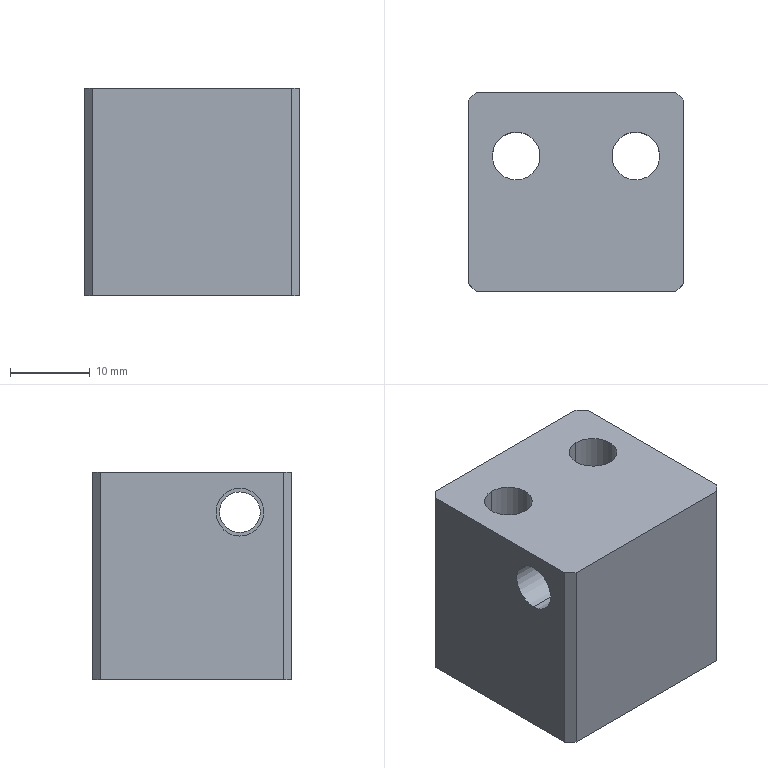Part | STEP file | J454-EBZ05-27-00-Part-1-2 | 1 solid | 36 faces | box 27 x 25 x 26 mm | volume 15181 mm3 | cylinder 18 | plane 14 | cone 4 | commonest cylinder face diameters 6 x8 2.5 x4 3 x4 5.1 x2
STEP:
#1=CARTESIAN_POINT('',(13.5,16.249,-3.3));
#2=VERTEX_POINT('',#1);
#3=CARTESIAN_POINT('',(14.75,17.,-3.3));
#4=VERTEX_POINT('',#3);
#5=CARTESIAN_POINT('',(14.75,17.,-3.3));
#6=DIRECTION('',(0.8572,0.515,0.));
#7=VECTOR('',#6,1000.);
#8=LINE('',#5,#7);
#9=EDGE_CURVE('',#2,#4,#8,.T.);
#10=ORIENTED_EDGE('',*,*,#9,.F.);
#11=CARTESIAN_POINT('',(12.25,17.,-3.3));
#12=VERTEX_POINT('',#11);
#13=CARTESIAN_POINT('',(12.25,17.,-3.3));
#14=DIRECTION('',(-0.8572,0.515,0.));
#15=VECTOR('',#14,1000.);
#16=LINE('',#13,#15);
#17=EDGE_CURVE('',#2,#12,#16,.T.);
#18=ORIENTED_EDGE('',*,*,#17,.T.);
#19=CARTESIAN_POINT('',(13.5,17.,-3.3));
#20=DIRECTION('',(0.,1.,0.));
#21=DIRECTION('',(1.,0.,0.));
#22=AXIS2_PLACEMENT_3D('',#19,#20,#21);
#23=CIRCLE('',#22,1.25);
#24=EDGE_CURVE('',#12,#4,#23,.T.);
#25=ORIENTED_EDGE('',*,*,#24,.T.);
#26=EDGE_LOOP('',(#10,#18,#25));
#27=FACE_OUTER_BOUND('',#26,.T.);
#28=CARTESIAN_POINT('',(13.5,17.,-3.3));
#29=DIRECTION('',(0.,1.,0.));
#30=DIRECTION('',(1.,0.,0.));
#31=AXIS2_PLACEMENT_3D('',#28,#29,#30);
#32=CONICAL_SURFACE('',#31,1.25,1.03);
#33=ADVANCED_FACE('',(#27),#32,.F.);
#34=ORIENTED_EDGE('',*,*,#24,.F.);
#35=CARTESIAN_POINT('',(12.25,19.,-3.3));
#36=VERTEX_POINT('',#35);
#37=CARTESIAN_POINT('',(12.25,25.,-3.3));
#38=DIRECTION('',(0.,1.,0.));
#39=VECTOR('',#38,1000.);
#40=LINE('',#37,#39);
#41=EDGE_CURVE('',#12,#36,#40,.T.);
#42=ORIENTED_EDGE('',*,*,#41,.T.);
#43=CARTESIAN_POINT('',(14.75,19.,-3.3));
#44=VERTEX_POINT('',#43);
#45=CARTESIAN_POINT('',(13.5,19.,-3.3));
#46=DIRECTION('',(0.,1.,0.));
#47=DIRECTION('',(1.,0.,0.));
#48=AXIS2_PLACEMENT_3D('',#45,#46,#47);
#49=CIRCLE('',#48,1.25);
#50=EDGE_CURVE('',#36,#44,#49,.T.);
#51=ORIENTED_EDGE('',*,*,#50,.T.);
#52=CARTESIAN_POINT('',(14.75,25.,-3.3));
#53=DIRECTION('',(0.,1.,0.));
#54=VECTOR('',#53,1000.);
#55=LINE('',#52,#54);
#56=EDGE_CURVE('',#4,#44,#55,.T.);
#57=ORIENTED_EDGE('',*,*,#56,.F.);
#58=EDGE_LOOP('',(#34,#42,#51,#57));
#59=FACE_OUTER_BOUND('',#58,.T.);
#60=CARTESIAN_POINT('',(13.5,25.,-3.3));
#61=DIRECTION('',(0.,1.,0.));
#62=DIRECTION('',(1.,0.,0.));
#63=AXIS2_PLACEMENT_3D('',#60,#61,#62);
#64=CYLINDRICAL_SURFACE('',#63,1.25);
#65=ADVANCED_FACE('',(#59),#64,.F.);
#66=CARTESIAN_POINT('',(12.,19.,-3.3));
#67=VERTEX_POINT('',#66);
#68=CARTESIAN_POINT('',(15.,19.,-3.3));
#69=VERTEX_POINT('',#68);
#70=CARTESIAN_POINT('',(13.5,19.,-3.3));
#71=DIRECTION('',(0.,1.,0.));
#72=DIRECTION('',(1.,0.,0.));
#73=AXIS2_PLACEMENT_3D('',#70,#71,#72);
#74=CIRCLE('',#73,1.5);
#75=EDGE_CURVE('',#67,#69,#74,.T.);
#76=ORIENTED_EDGE('',*,*,#75,.F.);
#77=CARTESIAN_POINT('',(12.,25.,-3.3));
#78=VERTEX_POINT('',#77);
#79=CARTESIAN_POINT('',(12.,25.,-3.3));
#80=DIRECTION('',(0.,1.,0.));
#81=VECTOR('',#80,1000.);
#82=LINE('',#79,#81);
#83=EDGE_CURVE('',#67,#78,#82,.T.);
#84=ORIENTED_EDGE('',*,*,#83,.T.);
#85=CARTESIAN_POINT('',(15.,25.,-3.3));
#86=VERTEX_POINT('',#85);
#87=CARTESIAN_POINT('',(13.5,25.,-3.3));
#88=DIRECTION('',(0.,1.,0.));
#89=DIRECTION('',(1.,0.,0.));
#90=AXIS2_PLACEMENT_3D('',#87,#88,#89);
#91=CIRCLE('',#90,1.5);
#92=EDGE_CURVE('',#78,#86,#91,.T.);
#93=ORIENTED_EDGE('',*,*,#92,.T.);
#94=CARTESIAN_POINT('',(15.,25.,-3.3));
#95=DIRECTION('',(0.,1.,0.));
#96=VECTOR('',#95,1000.);
#97=LINE('',#94,#96);
#98=EDGE_CURVE('',#69,#86,#97,.T.);
#99=ORIENTED_EDGE('',*,*,#98,.F.);
#100=EDGE_LOOP('',(#76,#84,#93,#99));
#101=FACE_OUTER_BOUND('',#100,.T.);
#102=CARTESIAN_POINT('',(13.5,25.,-3.3));
#103=DIRECTION('',(0.,1.,0.));
#104=DIRECTION('',(1.,0.,0.));
#105=AXIS2_PLACEMENT_3D('',#102,#103,#104);
#106=CYLINDRICAL_SURFACE('',#105,1.5);
#107=ADVANCED_FACE('',(#101),#106,.F.);
#108=CARTESIAN_POINT('',(13.5,16.249,9.3));
#109=VERTEX_POINT('',#108);
#110=CARTESIAN_POINT('',(14.75,17.,9.3));
#111=VERTEX_POINT('',#110);
#112=CARTESIAN_POINT('',(14.75,17.,9.3));
#113=DIRECTION('',(0.8572,0.515,0.));
#114=VECTOR('',#113,1000.);
#115=LINE('',#112,#114);
#116=EDGE_CURVE('',#109,#111,#115,.T.);
#117=ORIENTED_EDGE('',*,*,#116,.F.);
#118=CARTESIAN_POINT('',(12.25,17.,9.3));
#119=VERTEX_POINT('',#118);
#120=CARTESIAN_POINT('',(12.25,17.,9.3));
#121=DIRECTION('',(-0.8572,0.515,0.));
#122=VECTOR('',#121,1000.);
#123=LINE('',#120,#122);
#124=EDGE_CURVE('',#109,#119,#123,.T.);
#125=ORIENTED_EDGE('',*,*,#124,.T.);
#126=CARTESIAN_POINT('',(13.5,17.,9.3));
#127=DIRECTION('',(0.,1.,0.));
#128=DIRECTION('',(1.,0.,0.));
#129=AXIS2_PLACEMENT_3D('',#126,#127,#128);
#130=CIRCLE('',#129,1.25);
#131=EDGE_CURVE('',#119,#111,#130,.T.);
#132=ORIENTED_EDGE('',*,*,#131,.T.);
#133=EDGE_LOOP('',(#117,#125,#132));
#134=FACE_OUTER_BOUND('',#133,.T.);
#135=CARTESIAN_POINT('',(13.5,17.,9.3));
#136=DIRECTION('',(0.,1.,0.));
#137=DIRECTION('',(1.,0.,0.));
#138=AXIS2_PLACEMENT_3D('',#135,#136,#137);
#139=CONICAL_SURFACE('',#138,1.25,1.03);
#140=ADVANCED_FACE('',(#134),#139,.F.);
#141=ORIENTED_EDGE('',*,*,#131,.F.);
#142=CARTESIAN_POINT('',(12.25,19.,9.3));
#143=VERTEX_POINT('',#142);
#144=CARTESIAN_POINT('',(12.25,25.,9.3));
#145=DIRECTION('',(0.,1.,0.));
#146=VECTOR('',#145,1000.);
#147=LINE('',#144,#146);
#148=EDGE_CURVE('',#119,#143,#147,.T.);
#149=ORIENTED_EDGE('',*,*,#148,.T.);
#150=CARTESIAN_POINT('',(14.75,19.,9.3));
#151=VERTEX_POINT('',#150);
#152=CARTESIAN_POINT('',(13.5,19.,9.3));
#153=DIRECTION('',(0.,1.,0.));
#154=DIRECTION('',(1.,0.,0.));
#155=AXIS2_PLACEMENT_3D('',#152,#153,#154);
#156=CIRCLE('',#155,1.25);
#157=EDGE_CURVE('',#143,#151,#156,.T.);
#158=ORIENTED_EDGE('',*,*,#157,.T.);
#159=CARTESIAN_POINT('',(14.75,25.,9.3));
#160=DIRECTION('',(0.,1.,0.));
#161=VECTOR('',#160,1000.);
#162=LINE('',#159,#161);
#163=EDGE_CURVE('',#111,#151,#162,.T.);
#164=ORIENTED_EDGE('',*,*,#163,.F.);
#165=EDGE_LOOP('',(#141,#149,#158,#164));
#166=FACE_OUTER_BOUND('',#165,.T.);
#167=CARTESIAN_POINT('',(13.5,25.,9.3));
#168=DIRECTION('',(0.,1.,0.));
#169=DIRECTION('',(1.,0.,0.));
#170=AXIS2_PLACEMENT_3D('',#167,#168,#169);
#171=CYLINDRICAL_SURFACE('',#170,1.25);
#172=ADVANCED_FACE('',(#166),#171,.F.);
#173=CARTESIAN_POINT('',(12.,19.,9.3));
#174=VERTEX_POINT('',#173);
#175=CARTESIAN_POINT('',(15.,19.,9.3));
#176=VERTEX_POINT('',#175);
#177=CARTESIAN_POINT('',(13.5,19.,9.3));
#178=DIRECTION('',(0.,1.,0.));
#179=DIRECTION('',(1.,0.,0.));
#180=AXIS2_PLACEMENT_3D('',#177,#178,#179);
#181=CIRCLE('',#180,1.5);
#182=EDGE_CURVE('',#174,#176,#181,.T.);
#183=ORIENTED_EDGE('',*,*,#182,.F.);
#184=CARTESIAN_POINT('',(12.,25.,9.3));
#185=VERTEX_POINT('',#184);
#186=CARTESIAN_POINT('',(12.,25.,9.3));
#187=DIRECTION('',(0.,1.,0.));
#188=VECTOR('',#187,1000.);
#189=LINE('',#186,#188);
#190=EDGE_CURVE('',#174,#185,#189,.T.);
#191=ORIENTED_EDGE('',*,*,#190,.T.);
#192=CARTESIAN_POINT('',(15.,25.,9.3));
#193=VERTEX_POINT('',#192);
#194=CARTESIAN_POINT('',(13.5,25.,9.3));
#195=DIRECTION('',(0.,1.,0.));
#196=DIRECTION('',(1.,0.,0.));
#197=AXIS2_PLACEMENT_3D('',#194,#195,#196);
#198=CIRCLE('',#197,1.5);
#199=EDGE_CURVE('',#185,#193,#198,.T.);
#200=ORIENTED_EDGE('',*,*,#199,.T.);
#201=CARTESIAN_POINT('',(15.,25.,9.3));
#202=DIRECTION('',(0.,1.,0.));
#203=VECTOR('',#202,1000.);
#204=LINE('',#201,#203);
#205=EDGE_CURVE('',#176,#193,#204,.T.);
#206=ORIENTED_EDGE('',*,*,#205,.F.);
#207=EDGE_LOOP('',(#183,#191,#200,#206));
#208=FACE_OUTER_BOUND('',#207,.T.);
#209=CARTESIAN_POINT('',(13.5,25.,9.3));
#210=DIRECTION('',(0.,1.,0.));
#211=DIRECTION('',(1.,0.,0.));
#212=AXIS2_PLACEMENT_3D('',#209,#210,#211);
#213=CYLINDRICAL_SURFACE('',#212,1.5);
#214=ADVANCED_FACE('',(#208),#213,.F.);
#215=CARTESIAN_POINT('',(12.,6.5,8.));
#216=VERTEX_POINT('',#215);
#217=CARTESIAN_POINT('',(12.,6.5,14.));
#218=VERTEX_POINT('',#217);
#219=CARTESIAN_POINT('',(12.,6.5,11.));
#220=DIRECTION('',(-1.,0.,0.));
#221=DIRECTION('',(0.,0.,1.));
#222=AXIS2_PLACEMENT_3D('',#219,#220,#221);
#223=CIRCLE('',#222,3.);
#224=EDGE_CURVE('',#216,#218,#223,.T.);
#225=ORIENTED_EDGE('',*,*,#224,.F.);
#226=CARTESIAN_POINT('',(0.,6.5,8.));
#227=VERTEX_POINT('',#226);
#228=CARTESIAN_POINT('',(0.,6.5,8.));
#229=DIRECTION('',(-1.,0.,0.));
#230=VECTOR('',#229,1000.);
#231=LINE('',#228,#230);
#232=EDGE_CURVE('',#216,#227,#231,.T.);
#233=ORIENTED_EDGE('',*,*,#232,.T.);
#234=CARTESIAN_POINT('',(0.,6.5,14.));
#235=VERTEX_POINT('',#234);
#236=CARTESIAN_POINT('',(0.,6.5,11.));
#237=DIRECTION('',(-1.,0.,0.));
#238=DIRECTION('',(0.,0.,1.));
#239=AXIS2_PLACEMENT_3D('',#236,#237,#238);
#240=CIRCLE('',#239,3.);
#241=EDGE_CURVE('',#227,#235,#240,.T.);
#242=ORIENTED_EDGE('',*,*,#241,.T.);
#243=CARTESIAN_POINT('',(0.,6.5,14.));
#244=DIRECTION('',(-1.,0.,0.));
#245=VECTOR('',#244,1000.);
#246=LINE('',#243,#245);
#247=EDGE_CURVE('',#218,#235,#246,.T.);
#248=ORIENTED_EDGE('',*,*,#247,.F.);
#249=EDGE_LOOP('',(#225,#233,#242,#248));
#250=FACE_OUTER_BOUND('',#249,.T.);
#251=CARTESIAN_POINT('',(0.,6.5,11.));
#252=DIRECTION('',(-1.,0.,0.));
#253=DIRECTION('',(0.,0.,1.));
#254=AXIS2_PLACEMENT_3D('',#251,#252,#253);
#255=CYLINDRICAL_SURFACE('',#254,3.);
#256=ADVANCED_FACE('',(#250),#255,.F.);
#257=CARTESIAN_POINT('',(12.,6.5,13.55));
#258=VERTEX_POINT('',#257);
#259=CARTESIAN_POINT('',(12.,6.5,8.45));
#260=VERTEX_POINT('',#259);
#261=CARTESIAN_POINT('',(12.,6.5,11.));
#262=DIRECTION('',(-1.,0.,0.));
#263=DIRECTION('',(0.,0.,1.));
#264=AXIS2_PLACEMENT_3D('',#261,#262,#263);
#265=CIRCLE('',#264,2.55);
#266=EDGE_CURVE('',#258,#260,#265,.T.);
#267=ORIENTED_EDGE('',*,*,#266,.T.);
#268=CARTESIAN_POINT('',(15.,6.5,8.45));
#269=VERTEX_POINT('',#268);
#270=CARTESIAN_POINT('',(27.,6.5,8.45));
#271=DIRECTION('',(1.,0.,0.));
#272=VECTOR('',#271,1000.);
#273=LINE('',#270,#272);
#274=EDGE_CURVE('',#260,#269,#273,.T.);
#275=ORIENTED_EDGE('',*,*,#274,.T.);
#276=CARTESIAN_POINT('',(15.,6.5,13.55));
#277=VERTEX_POINT('',#276);
#278=CARTESIAN_POINT('',(15.,6.5,11.));
#279=DIRECTION('',(1.,0.,0.));
#280=DIRECTION('',(0.,0.,1.));
#281=AXIS2_PLACEMENT_3D('',#278,#279,#280);
#282=CIRCLE('',#281,2.55);
#283=EDGE_CURVE('',#269,#277,#282,.T.);
#284=ORIENTED_EDGE('',*,*,#283,.T.);
#285=CARTESIAN_POINT('',(27.,6.5,13.55));
#286=DIRECTION('',(1.,0.,0.));
#287=VECTOR('',#286,1000.);
#288=LINE('',#285,#287);
#289=EDGE_CURVE('',#258,#277,#288,.T.);
#290=ORIENTED_EDGE('',*,*,#289,.F.);
#291=EDGE_LOOP('',(#267,#275,#284,#290));
#292=FACE_OUTER_BOUND('',#291,.T.);
#293=CARTESIAN_POINT('',(27.,6.5,11.));
#294=DIRECTION('',(1.,0.,0.));
#295=DIRECTION('',(0.,0.,1.));
#296=AXIS2_PLACEMENT_3D('',#293,#294,#295);
#297=CYLINDRICAL_SURFACE('',#296,2.55);
#298=ADVANCED_FACE('',(#292),#297,.F.);
#299=CARTESIAN_POINT('',(15.,6.5,8.));
#300=VERTEX_POINT('',#299);
#301=CARTESIAN_POINT('',(15.,6.5,14.));
#302=VERTEX_POINT('',#301);
#303=CARTESIAN_POINT('',(15.,6.5,11.));
#304=DIRECTION('',(1.,0.,0.));
#305=DIRECTION('',(0.,0.,1.));
#306=AXIS2_PLACEMENT_3D('',#303,#304,#305);
#307=CIRCLE('',#306,3.);
#308=EDGE_CURVE('',#300,#302,#307,.T.);
#309=ORIENTED_EDGE('',*,*,#308,.F.);
#310=CARTESIAN_POINT('',(27.,6.5,8.));
#311=VERTEX_POINT('',#310);
#312=CARTESIAN_POINT('',(27.,6.5,8.));
#313=DIRECTION('',(1.,0.,0.));
#314=VECTOR('',#313,1000.);
#315=LINE('',#312,#314);
#316=EDGE_CURVE('',#300,#311,#315,.T.);
#317=ORIENTED_EDGE('',*,*,#316,.T.);
#318=CARTESIAN_POINT('',(27.,6.5,14.));
#319=VERTEX_POINT('',#318);
#320=CARTESIAN_POINT('',(27.,6.5,11.));
#321=DIRECTION('',(1.,0.,0.));
#322=DIRECTION('',(0.,0.,1.));
#323=AXIS2_PLACEMENT_3D('',#320,#321,#322);
#324=CIRCLE('',#323,3.);
#325=EDGE_CURVE('',#311,#319,#324,.T.);
#326=ORIENTED_EDGE('',*,*,#325,.T.);
#327=CARTESIAN_POINT('',(27.,6.5,14.));
#328=DIRECTION('',(1.,0.,0.));
#329=VECTOR('',#328,1000.);
#330=LINE('',#327,#329);
#331=EDGE_CURVE('',#302,#319,#330,.T.);
#332=ORIENTED_EDGE('',*,*,#331,.F.);
#333=EDGE_LOOP('',(#309,#317,#326,#332));
#334=FACE_OUTER_BOUND('',#333,.T.);
#335=CARTESIAN_POINT('',(27.,6.5,11.));
#336=DIRECTION('',(1.,0.,0.));
#337=DIRECTION('',(0.,0.,1.));
#338=AXIS2_PLACEMENT_3D('',#335,#336,#337);
#339=CYLINDRICAL_SURFACE('',#338,3.);
#340=ADVANCED_FACE('',(#334),#339,.F.);
#341=CARTESIAN_POINT('',(6.,20.,16.));
#342=VERTEX_POINT('',#341);
#343=CARTESIAN_POINT('',(6.,14.,16.));
#344=VERTEX_POINT('',#343);
#345=CARTESIAN_POINT('',(6.,17.,16.));
#346=DIRECTION('',(0.,0.,-1.));
#347=DIRECTION('',(0.,-1.,0.));
#348=AXIS2_PLACEMENT_3D('',#345,#346,#347);
#349=CIRCLE('',#348,3.);
#350=EDGE_CURVE('',#342,#344,#349,.T.);
#351=ORIENTED_EDGE('',*,*,#350,.F.);
#352=CARTESIAN_POINT('',(6.,20.,-10.));
#353=VERTEX_POINT('',#352);
#354=CARTESIAN_POINT('',(6.,20.,16.));
#355=DIRECTION('',(0.,0.,-1.));
#356=VECTOR('',#355,1000.);
#357=LINE('',#354,#356);
#358=EDGE_CURVE('',#342,#353,#357,.T.);
#359=ORIENTED_EDGE('',*,*,#358,.T.);
#360=CARTESIAN_POINT('',(6.,14.,-10.));
#361=VERTEX_POINT('',#360);
#362=CARTESIAN_POINT('',(6.,17.,-10.));
#363=DIRECTION('',(0.,0.,1.));
#364=DIRECTION('',(0.,1.,0.));
#365=AXIS2_PLACEMENT_3D('',#362,#363,#364);
#366=CIRCLE('',#365,3.);
#367=EDGE_CURVE('',#361,#353,#366,.T.);
#368=ORIENTED_EDGE('',*,*,#367,.F.);
#369=CARTESIAN_POINT('',(6.,14.,16.));
#370=DIRECTION('',(0.,0.,-1.));
#371=VECTOR('',#370,1000.);
#372=LINE('',#369,#371);
#373=EDGE_CURVE('',#344,#361,#372,.T.);
#374=ORIENTED_EDGE('',*,*,#373,.F.);
#375=EDGE_LOOP('',(#351,#359,#368,#374));
#376=FACE_OUTER_BOUND('',#375,.T.);
#377=CARTESIAN_POINT('',(6.,17.,16.));
#378=DIRECTION('',(0.,0.,-1.));
#379=DIRECTION('',(0.,-1.,0.));
#380=AXIS2_PLACEMENT_3D('',#377,#378,#379);
#381=CYLINDRICAL_SURFACE('',#380,3.);
#382=ADVANCED_FACE('',(#376),#381,.F.);
#383=CARTESIAN_POINT('',(21.,20.,16.));
#384=VERTEX_POINT('',#383);
#385=CARTESIAN_POINT('',(21.,14.,16.));
#386=VERTEX_POINT('',#385);
#387=CARTESIAN_POINT('',(21.,17.,16.));
#388=DIRECTION('',(0.,0.,-1.));
#389=DIRECTION('',(0.,-1.,0.));
#390=AXIS2_PLACEMENT_3D('',#387,#388,#389);
#391=CIRCLE('',#390,3.);
#392=EDGE_CURVE('',#384,#386,#391,.T.);
#393=ORIENTED_EDGE('',*,*,#392,.F.);
#394=CARTESIAN_POINT('',(21.,20.,-10.));
#395=VERTEX_POINT('',#394);
#396=CARTESIAN_POINT('',(21.,20.,16.));
#397=DIRECTION('',(0.,0.,-1.));
#398=VECTOR('',#397,1000.);
#399=LINE('',#396,#398);
#400=EDGE_CURVE('',#384,#395,#399,.T.);
#401=ORIENTED_EDGE('',*,*,#400,.T.);
#402=CARTESIAN_POINT('',(21.,14.,-10.));
#403=VERTEX_POINT('',#402);
#404=CARTESIAN_POINT('',(21.,17.,-10.));
#405=DIRECTION('',(0.,0.,1.));
#406=DIRECTION('',(0.,1.,0.));
#407=AXIS2_PLACEMENT_3D('',#404,#405,#406);
#408=CIRCLE('',#407,3.);
#409=EDGE_CURVE('',#403,#395,#408,.T.);
#410=ORIENTED_EDGE('',*,*,#409,.F.);
#411=CARTESIAN_POINT('',(21.,14.,16.));
#412=DIRECTION('',(0.,0.,-1.));
#413=VECTOR('',#412,1000.);
#414=LINE('',#411,#413);
#415=EDGE_CURVE('',#386,#403,#414,.T.);
#416=ORIENTED_EDGE('',*,*,#415,.F.);
#417=EDGE_LOOP('',(#393,#401,#410,#416));
#418=FACE_OUTER_BOUND('',#417,.T.);
#419=CARTESIAN_POINT('',(21.,17.,16.));
#420=DIRECTION('',(0.,0.,-1.));
#421=DIRECTION('',(0.,-1.,0.));
#422=AXIS2_PLACEMENT_3D('',#419,#420,#421);
#423=CYLINDRICAL_SURFACE('',#422,3.);
#424=ADVANCED_FACE('',(#418),#423,.F.);
#425=CARTESIAN_POINT('',(6.,17.,16.));
#426=DIRECTION('',(0.,0.,-1.));
#427=DIRECTION('',(0.,-1.,0.));
#428=AXIS2_PLACEMENT_3D('',#425,#426,#427);
#429=CIRCLE('',#428,3.);
#430=EDGE_CURVE('',#344,#342,#429,.T.);
#431=ORIENTED_EDGE('',*,*,#430,.T.);
#432=ORIENTED_EDGE('',*,*,#350,.T.);
#433=EDGE_LOOP('',(#431,#432));
#434=FACE_BOUND('',#433,.T.);
#435=CARTESIAN_POINT('',(21.,17.,16.));
#436=DIRECTION('',(0.,0.,-1.));
#437=DIRECTION('',(0.,-1.,0.));
#438=AXIS2_PLACEMENT_3D('',#435,#436,#437);
#439=CIRCLE('',#438,3.);
#440=EDGE_CURVE('',#386,#384,#439,.T.);
#441=ORIENTED_EDGE('',*,*,#440,.T.);
#442=ORIENTED_EDGE('',*,*,#392,.T.);
#443=EDGE_LOOP('',(#441,#442));
#444=FACE_BOUND('',#443,.T.);
#445=CARTESIAN_POINT('',(26.,0.,16.));
#446=VERTEX_POINT('',#445);
#447=CARTESIAN_POINT('',(1.,0.,16.));
#448=VERTEX_POINT('',#447);
#449=CARTESIAN_POINT('',(13.5,0.,16.));
#450=DIRECTION('',(-1.,0.,0.));
#451=VECTOR('',#450,1000.);
#452=LINE('',#449,#451);
#453=EDGE_CURVE('',#446,#448,#452,.T.);
#454=ORIENTED_EDGE('',*,*,#453,.F.);
#455=CARTESIAN_POINT('',(27.,1.,16.));
#456=VERTEX_POINT('',#455);
#457=CARTESIAN_POINT('',(26.,0.,16.));
#458=DIRECTION('',(0.7071,0.7071,0.));
#459=VECTOR('',#458,1000.);
#460=LINE('',#457,#459);
#461=EDGE_CURVE('',#446,#456,#460,.T.);
#462=ORIENTED_EDGE('',*,*,#461,.T.);
#463=CARTESIAN_POINT('',(27.,24.,16.));
#464=VERTEX_POINT('',#463);
#465=CARTESIAN_POINT('',(27.,12.5,16.));
#466=DIRECTION('',(0.,-1.,0.));
#467=VECTOR('',#466,1000.);
#468=LINE('',#465,#467);
#469=EDGE_CURVE('',#464,#456,#468,.T.);
#470=ORIENTED_EDGE('',*,*,#469,.F.);
#471=CARTESIAN_POINT('',(26.,25.,16.));
#472=VERTEX_POINT('',#471);
#473=CARTESIAN_POINT('',(26.,25.,16.));
#474=DIRECTION('',(-0.7071,0.7071,0.));
#475=VECTOR('',#474,1000.);
#476=LINE('',#473,#475);
#477=EDGE_CURVE('',#464,#472,#476,.T.);
#478=ORIENTED_EDGE('',*,*,#477,.T.);
#479=CARTESIAN_POINT('',(1.,25.,16.));
#480=VERTEX_POINT('',#479);
#481=CARTESIAN_POINT('',(13.5,25.,16.));
#482=DIRECTION('',(1.,0.,0.));
#483=VECTOR('',#482,1000.);
#484=LINE('',#481,#483);
#485=EDGE_CURVE('',#480,#472,#484,.T.);
#486=ORIENTED_EDGE('',*,*,#485,.F.);
#487=CARTESIAN_POINT('',(0.,24.,16.));
#488=VERTEX_POINT('',#487);
#489=CARTESIAN_POINT('',(1.,25.,16.));
#490=DIRECTION('',(-0.7071,-0.7071,0.));
#491=VECTOR('',#490,1000.);
#492=LINE('',#489,#491);
#493=EDGE_CURVE('',#480,#488,#492,.T.);
#494=ORIENTED_EDGE('',*,*,#493,.T.);
#495=CARTESIAN_POINT('',(0.,1.,16.));
#496=VERTEX_POINT('',#495);
#497=CARTESIAN_POINT('',(0.,12.5,16.));
#498=DIRECTION('',(0.,1.,0.));
#499=VECTOR('',#498,1000.);
#500=LINE('',#497,#499);
#501=EDGE_CURVE('',#496,#488,#500,.T.);
#502=ORIENTED_EDGE('',*,*,#501,.F.);
#503=CARTESIAN_POINT('',(1.,0.,16.));
#504=DIRECTION('',(0.7071,-0.7071,0.));
#505=VECTOR('',#504,1000.);
#506=LINE('',#503,#505);
#507=EDGE_CURVE('',#496,#448,#506,.T.);
#508=ORIENTED_EDGE('',*,*,#507,.T.);
#509=EDGE_LOOP('',(#454,#462,#470,#478,#486,#494,#502,#508));
#510=FACE_OUTER_BOUND('',#509,.T.);
#511=CARTESIAN_POINT('',(13.5,12.5,16.));
#512=DIRECTION('',(0.,0.,1.));
#513=DIRECTION('',(0.,1.,0.));
#514=AXIS2_PLACEMENT_3D('',#511,#512,#513);
#515=PLANE('',#514);
#516=ADVANCED_FACE('',(#434,#444,#510),#515,.T.);
#517=CARTESIAN_POINT('',(27.,6.5,11.));
#518=DIRECTION('',(1.,0.,0.));
#519=DIRECTION('',(0.,0.,1.));
#520=AXIS2_PLACEMENT_3D('',#517,#518,#519);
#521=CIRCLE('',#520,3.);
#522=EDGE_CURVE('',#319,#311,#521,.T.);
#523=ORIENTED_EDGE('',*,*,#522,.F.);
#524=ORIENTED_EDGE('',*,*,#325,.F.);
#525=EDGE_LOOP('',(#523,#524));
#526=FACE_BOUND('',#525,.T.);
#527=ORIENTED_EDGE('',*,*,#469,.T.);
#528=CARTESIAN_POINT('',(27.,1.,-10.));
#529=VERTEX_POINT('',#528);
#530=CARTESIAN_POINT('',(27.,1.,-10.));
#531=DIRECTION('',(0.,0.,-1.));
#532=VECTOR('',#531,1000.);
#533=LINE('',#530,#532);
#534=EDGE_CURVE('',#456,#529,#533,.T.);
#535=ORIENTED_EDGE('',*,*,#534,.T.);
#536=CARTESIAN_POINT('',(27.,24.,-10.));
#537=VERTEX_POINT('',#536);
#538=CARTESIAN_POINT('',(27.,12.5,-10.));
#539=DIRECTION('',(0.,1.,0.));
#540=VECTOR('',#539,1000.);
#541=LINE('',#538,#540);
#542=EDGE_CURVE('',#529,#537,#541,.T.);
#543=ORIENTED_EDGE('',*,*,#542,.T.);
#544=CARTESIAN_POINT('',(27.,24.,-10.));
#545=DIRECTION('',(0.,0.,1.));
#546=VECTOR('',#545,1000.);
#547=LINE('',#544,#546);
#548=EDGE_CURVE('',#537,#464,#547,.T.);
#549=ORIENTED_EDGE('',*,*,#548,.T.);
#550=EDGE_LOOP('',(#527,#535,#543,#549));
#551=FACE_OUTER_BOUND('',#550,.T.);
#552=CARTESIAN_POINT('',(27.,12.5,-10.));
#553=DIRECTION('',(1.,0.,0.));
#554=DIRECTION('',(0.,0.,-1.));
#555=AXIS2_PLACEMENT_3D('',#552,#553,#554);
#556=PLANE('',#555);
#557=ADVANCED_FACE('',(#526,#551),#556,.T.);
#558=CARTESIAN_POINT('',(1.,0.,-10.));
#559=VERTEX_POINT('',#558);
#560=CARTESIAN_POINT('',(26.,0.,-10.));
#561=VERTEX_POINT('',#560);
#562=CARTESIAN_POINT('',(13.5,0.,-10.));
#563=DIRECTION('',(1.,0.,0.));
#564=VECTOR('',#563,1000.);
#565=LINE('',#562,#564);
#566=EDGE_CURVE('',#559,#561,#565,.T.);
#567=ORIENTED_EDGE('',*,*,#566,.T.);
#568=CARTESIAN_POINT('',(26.,0.,-10.));
#569=DIRECTION('',(0.,0.,1.));
#570=VECTOR('',#569,1000.);
#571=LINE('',#568,#570);
#572=EDGE_CURVE('',#561,#446,#571,.T.);
#573=ORIENTED_EDGE('',*,*,#572,.T.);
#574=ORIENTED_EDGE('',*,*,#453,.T.);
#575=CARTESIAN_POINT('',(1.,0.,-10.));
#576=DIRECTION('',(0.,0.,-1.));
#577=VECTOR('',#576,1000.);
#578=LINE('',#575,#577);
#579=EDGE_CURVE('',#448,#559,#578,.T.);
#580=ORIENTED_EDGE('',*,*,#579,.T.);
#581=EDGE_LOOP('',(#567,#573,#574,#580));
#582=FACE_OUTER_BOUND('',#581,.T.);
#583=CARTESIAN_POINT('',(13.5,0.,-10.));
#584=DIRECTION('',(0.,-1.,0.));
#585=DIRECTION('',(0.,0.,1.));
#586=AXIS2_PLACEMENT_3D('',#583,#584,#585);
#587=PLANE('',#586);
#588=ADVANCED_FACE('',(#582),#587,.T.);
#589=CARTESIAN_POINT('',(0.,6.5,11.));
#590=DIRECTION('',(-1.,0.,0.));
#591=DIRECTION('',(0.,0.,1.));
#592=AXIS2_PLACEMENT_3D('',#589,#590,#591);
#593=CIRCLE('',#592,3.);
#594=EDGE_CURVE('',#235,#227,#593,.T.);
#595=ORIENTED_EDGE('',*,*,#594,.F.);
#596=ORIENTED_EDGE('',*,*,#241,.F.);
#597=EDGE_LOOP('',(#595,#596));
#598=FACE_BOUND('',#597,.T.);
#599=CARTESIAN_POINT('',(0.,24.,-10.));
#600=VERTEX_POINT('',#599);
#601=CARTESIAN_POINT('',(0.,1.,-10.));
#602=VERTEX_POINT('',#601);
#603=CARTESIAN_POINT('',(0.,12.5,-10.));
#604=DIRECTION('',(0.,-1.,0.));
#605=VECTOR('',#604,1000.);
#606=LINE('',#603,#605);
#607=EDGE_CURVE('',#600,#602,#606,.T.);
#608=ORIENTED_EDGE('',*,*,#607,.T.);
#609=CARTESIAN_POINT('',(0.,1.,-10.));
#610=DIRECTION('',(0.,0.,1.));
#611=VECTOR('',#610,1000.);
#612=LINE('',#609,#611);
#613=EDGE_CURVE('',#602,#496,#612,.T.);
#614=ORIENTED_EDGE('',*,*,#613,.T.);
#615=ORIENTED_EDGE('',*,*,#501,.T.);
#616=CARTESIAN_POINT('',(0.,24.,-10.));
#617=DIRECTION('',(0.,0.,-1.));
#618=VECTOR('',#617,1000.);
#619=LINE('',#616,#618);
#620=EDGE_CURVE('',#488,#600,#619,.T.);
#621=ORIENTED_EDGE('',*,*,#620,.T.);
#622=EDGE_LOOP('',(#608,#614,#615,#621));
#623=FACE_OUTER_BOUND('',#622,.T.);
#624=CARTESIAN_POINT('',(0.,12.5,-10.));
#625=DIRECTION('',(-1.,0.,0.));
#626=DIRECTION('',(0.,0.,1.));
#627=AXIS2_PLACEMENT_3D('',#624,#625,#626);
#628=PLANE('',#627);
#629=ADVANCED_FACE('',(#598,#623),#628,.T.);
#630=ORIENTED_EDGE('',*,*,#367,.T.);
#631=CARTESIAN_POINT('',(6.,17.,-10.));
#632=DIRECTION('',(0.,0.,1.));
#633=DIRECTION('',(0.,1.,0.));
#634=AXIS2_PLACEMENT_3D('',#631,#632,#633);
#635=CIRCLE('',#634,3.);
#636=EDGE_CURVE('',#353,#361,#635,.T.);
#637=ORIENTED_EDGE('',*,*,#636,.T.);
#638=EDGE_LOOP('',(#630,#637));
#639=FACE_BOUND('',#638,.T.);
#640=ORIENTED_EDGE('',*,*,#409,.T.);
#641=CARTESIAN_POINT('',(21.,17.,-10.));
#642=DIRECTION('',(0.,0.,1.));
#643=DIRECTION('',(0.,1.,0.));
#644=AXIS2_PLACEMENT_3D('',#641,#642,#643);
#645=CIRCLE('',#644,3.);
#646=EDGE_CURVE('',#395,#403,#645,.T.);
#647=ORIENTED_EDGE('',*,*,#646,.T.);
#648=EDGE_LOOP('',(#640,#647));
#649=FACE_BOUND('',#648,.T.);
#650=ORIENTED_EDGE('',*,*,#542,.F.);
#651=CARTESIAN_POINT('',(26.,0.,-10.));
#652=DIRECTION('',(-0.7071,-0.7071,0.));
#653=VECTOR('',#652,1000.);
#654=LINE('',#651,#653);
#655=EDGE_CURVE('',#529,#561,#654,.T.);
#656=ORIENTED_EDGE('',*,*,#655,.T.);
#657=ORIENTED_EDGE('',*,*,#566,.F.);
#658=CARTESIAN_POINT('',(1.,0.,-10.));
#659=DIRECTION('',(-0.7071,0.7071,0.));
#660=VECTOR('',#659,1000.);
#661=LINE('',#658,#660);
#662=EDGE_CURVE('',#559,#602,#661,.T.);
#663=ORIENTED_EDGE('',*,*,#662,.T.);
#664=ORIENTED_EDGE('',*,*,#607,.F.);
#665=CARTESIAN_POINT('',(1.,25.,-10.));
#666=VERTEX_POINT('',#665);
#667=CARTESIAN_POINT('',(1.,25.,-10.));
#668=DIRECTION('',(0.7071,0.7071,0.));
#669=VECTOR('',#668,1000.);
#670=LINE('',#667,#669);
#671=EDGE_CURVE('',#600,#666,#670,.T.);
#672=ORIENTED_EDGE('',*,*,#671,.T.);
#673=CARTESIAN_POINT('',(26.,25.,-10.));
#674=VERTEX_POINT('',#673);
#675=CARTESIAN_POINT('',(13.5,25.,-10.));
#676=DIRECTION('',(-1.,0.,0.));
#677=VECTOR('',#676,1000.);
#678=LINE('',#675,#677);
#679=EDGE_CURVE('',#674,#666,#678,.T.);
#680=ORIENTED_EDGE('',*,*,#679,.F.);
#681=CARTESIAN_POINT('',(26.,25.,-10.));
#682=DIRECTION('',(0.7071,-0.7071,0.));
#683=VECTOR('',#682,1000.);
#684=LINE('',#681,#683);
#685=EDGE_CURVE('',#674,#537,#684,.T.);
#686=ORIENTED_EDGE('',*,*,#685,.T.);
#687=EDGE_LOOP('',(#650,#656,#657,#663,#664,#672,#680,#686));
#688=FACE_OUTER_BOUND('',#687,.T.);
#689=CARTESIAN_POINT('',(13.5,12.5,-10.));
#690=DIRECTION('',(0.,0.,-1.));
#691=DIRECTION('',(0.,-1.,0.));
#692=AXIS2_PLACEMENT_3D('',#689,#690,#691);
#693=PLANE('',#692);
#694=ADVANCED_FACE('',(#639,#649,#688),#693,.T.);
#695=CARTESIAN_POINT('',(13.5,25.,-3.3));
#696=DIRECTION('',(0.,1.,0.));
#697=DIRECTION('',(1.,0.,0.));
#698=AXIS2_PLACEMENT_3D('',#695,#696,#697);
#699=CIRCLE('',#698,1.5);
#700=EDGE_CURVE('',#86,#78,#699,.T.);
#701=ORIENTED_EDGE('',*,*,#700,.F.);
#702=ORIENTED_EDGE('',*,*,#92,.F.);
#703=EDGE_LOOP('',(#701,#702));
#704=FACE_BOUND('',#703,.T.);
#705=CARTESIAN_POINT('',(13.5,25.,9.3));
#706=DIRECTION('',(0.,1.,0.));
#707=DIRECTION('',(1.,0.,0.));
#708=AXIS2_PLACEMENT_3D('',#705,#706,#707);
#709=CIRCLE('',#708,1.5);
#710=EDGE_CURVE('',#193,#185,#709,.T.);
#711=ORIENTED_EDGE('',*,*,#710,.F.);
#712=ORIENTED_EDGE('',*,*,#199,.F.);
#713=EDGE_LOOP('',(#711,#712));
#714=FACE_BOUND('',#713,.T.);
#715=ORIENTED_EDGE('',*,*,#679,.T.);
#716=CARTESIAN_POINT('',(1.,25.,-10.));
#717=DIRECTION('',(0.,0.,1.));
#718=VECTOR('',#717,1000.);
#719=LINE('',#716,#718);
#720=EDGE_CURVE('',#666,#480,#719,.T.);
#721=ORIENTED_EDGE('',*,*,#720,.T.);
#722=ORIENTED_EDGE('',*,*,#485,.T.);
#723=CARTESIAN_POINT('',(26.,25.,-10.));
#724=DIRECTION('',(0.,0.,-1.));
#725=VECTOR('',#724,1000.);
#726=LINE('',#723,#725);
#727=EDGE_CURVE('',#472,#674,#726,.T.);
#728=ORIENTED_EDGE('',*,*,#727,.T.);
#729=EDGE_LOOP('',(#715,#721,#722,#728));
#730=FACE_OUTER_BOUND('',#729,.T.);
#731=CARTESIAN_POINT('',(13.5,25.,-10.));
#732=DIRECTION('',(0.,1.,0.));
#733=DIRECTION('',(0.,0.,-1.));
#734=AXIS2_PLACEMENT_3D('',#731,#732,#733);
#735=PLANE('',#734);
#736=ADVANCED_FACE('',(#704,#714,#730),#735,.T.);
#737=ORIENTED_EDGE('',*,*,#400,.F.);
#738=ORIENTED_EDGE('',*,*,#440,.F.);
#739=ORIENTED_EDGE('',*,*,#415,.T.);
#740=ORIENTED_EDGE('',*,*,#646,.F.);
#741=EDGE_LOOP('',(#737,#738,#739,#740));
#742=FACE_OUTER_BOUND('',#741,.T.);
#743=CARTESIAN_POINT('',(21.,17.,16.));
#744=DIRECTION('',(0.,0.,-1.));
#745=DIRECTION('',(0.,-1.,0.));
#746=AXIS2_PLACEMENT_3D('',#743,#744,#745);
#747=CYLINDRICAL_SURFACE('',#746,3.);
#748=ADVANCED_FACE('',(#742),#747,.F.);
#749=ORIENTED_EDGE('',*,*,#358,.F.);
#750=ORIENTED_EDGE('',*,*,#430,.F.);
#751=ORIENTED_EDGE('',*,*,#373,.T.);
#752=ORIENTED_EDGE('',*,*,#636,.F.);
#753=EDGE_LOOP('',(#749,#750,#751,#752));
#754=FACE_OUTER_BOUND('',#753,.T.);
#755=CARTESIAN_POINT('',(6.,17.,16.));
#756=DIRECTION('',(0.,0.,-1.));
#757=DIRECTION('',(0.,-1.,0.));
#758=AXIS2_PLACEMENT_3D('',#755,#756,#757);
#759=CYLINDRICAL_SURFACE('',#758,3.);
#760=ADVANCED_FACE('',(#754),#759,.F.);
#761=ORIENTED_EDGE('',*,*,#685,.F.);
#762=ORIENTED_EDGE('',*,*,#727,.F.);
#763=ORIENTED_EDGE('',*,*,#477,.F.);
#764=ORIENTED_EDGE('',*,*,#548,.F.);
#765=EDGE_LOOP('',(#761,#762,#763,#764));
#766=FACE_OUTER_BOUND('',#765,.T.);
#767=CARTESIAN_POINT('',(27.,24.,-10.));
#768=DIRECTION('',(-0.7071,-0.7071,0.));
#769=DIRECTION('',(0.,0.,1.));
#770=AXIS2_PLACEMENT_3D('',#767,#768,#769);
#771=PLANE('',#770);
#772=ADVANCED_FACE('',(#766),#771,.F.);
#773=ORIENTED_EDGE('',*,*,#671,.F.);
#774=ORIENTED_EDGE('',*,*,#620,.F.);
#775=ORIENTED_EDGE('',*,*,#493,.F.);
#776=ORIENTED_EDGE('',*,*,#720,.F.);
#777=EDGE_LOOP('',(#773,#774,#775,#776));
#778=FACE_OUTER_BOUND('',#777,.T.);
#779=CARTESIAN_POINT('',(1.,25.,-10.));
#780=DIRECTION('',(0.7071,-0.7071,0.));
#781=DIRECTION('',(0.,0.,1.));
#782=AXIS2_PLACEMENT_3D('',#779,#780,#781);
#783=PLANE('',#782);
#784=ADVANCED_FACE('',(#778),#783,.F.);
#785=ORIENTED_EDGE('',*,*,#662,.F.);
#786=ORIENTED_EDGE('',*,*,#579,.F.);
#787=ORIENTED_EDGE('',*,*,#507,.F.);
#788=ORIENTED_EDGE('',*,*,#613,.F.);
#789=EDGE_LOOP('',(#785,#786,#787,#788));
#790=FACE_OUTER_BOUND('',#789,.T.);
#791=CARTESIAN_POINT('',(0.,1.,-10.));
#792=DIRECTION('',(0.7071,0.7071,0.));
#793=DIRECTION('',(0.,0.,1.));
#794=AXIS2_PLACEMENT_3D('',#791,#792,#793);
#795=PLANE('',#794);
#796=ADVANCED_FACE('',(#790),#795,.F.);
#797=ORIENTED_EDGE('',*,*,#655,.F.);
#798=ORIENTED_EDGE('',*,*,#534,.F.);
#799=ORIENTED_EDGE('',*,*,#461,.F.);
#800=ORIENTED_EDGE('',*,*,#572,.F.);
#801=EDGE_LOOP('',(#797,#798,#799,#800));
#802=FACE_OUTER_BOUND('',#801,.T.);
#803=CARTESIAN_POINT('',(26.,0.,-10.));
#804=DIRECTION('',(-0.7071,0.7071,0.));
#805=DIRECTION('',(0.,0.,1.));
#806=AXIS2_PLACEMENT_3D('',#803,#804,#805);
#807=PLANE('',#806);
#808=ADVANCED_FACE('',(#802),#807,.F.);
#809=ORIENTED_EDGE('',*,*,#316,.F.);
#810=CARTESIAN_POINT('',(15.,6.5,11.));
#811=DIRECTION('',(1.,0.,0.));
#812=DIRECTION('',(0.,0.,1.));
#813=AXIS2_PLACEMENT_3D('',#810,#811,#812);
#814=CIRCLE('',#813,3.);
#815=EDGE_CURVE('',#302,#300,#814,.T.);
#816=ORIENTED_EDGE('',*,*,#815,.F.);
#817=ORIENTED_EDGE('',*,*,#331,.T.);
#818=ORIENTED_EDGE('',*,*,#522,.T.);
#819=EDGE_LOOP('',(#809,#816,#817,#818));
#820=FACE_OUTER_BOUND('',#819,.T.);
#821=CARTESIAN_POINT('',(27.,6.5,11.));
#822=DIRECTION('',(1.,0.,0.));
#823=DIRECTION('',(0.,0.,1.));
#824=AXIS2_PLACEMENT_3D('',#821,#822,#823);
#825=CYLINDRICAL_SURFACE('',#824,3.);
#826=ADVANCED_FACE('',(#820),#825,.F.);
#827=CARTESIAN_POINT('',(15.,6.5,11.));
#828=DIRECTION('',(1.,0.,0.));
#829=DIRECTION('',(0.,0.,1.));
#830=AXIS2_PLACEMENT_3D('',#827,#828,#829);
#831=CIRCLE('',#830,2.55);
#832=EDGE_CURVE('',#277,#269,#831,.T.);
#833=ORIENTED_EDGE('',*,*,#832,.F.);
#834=ORIENTED_EDGE('',*,*,#283,.F.);
#835=EDGE_LOOP('',(#833,#834));
#836=FACE_BOUND('',#835,.T.);
#837=ORIENTED_EDGE('',*,*,#815,.T.);
#838=ORIENTED_EDGE('',*,*,#308,.T.);
#839=EDGE_LOOP('',(#837,#838));
#840=FACE_OUTER_BOUND('',#839,.T.);
#841=CARTESIAN_POINT('',(15.,6.5,8.));
#842=DIRECTION('',(-1.,0.,0.));
#843=DIRECTION('',(0.,0.,-1.));
#844=AXIS2_PLACEMENT_3D('',#841,#842,#843);
#845=PLANE('',#844);
#846=ADVANCED_FACE('',(#836,#840),#845,.F.);
#847=ORIENTED_EDGE('',*,*,#274,.F.);
#848=CARTESIAN_POINT('',(12.,6.5,11.));
#849=DIRECTION('',(-1.,0.,0.));
#850=DIRECTION('',(0.,0.,1.));
#851=AXIS2_PLACEMENT_3D('',#848,#849,#850);
#852=CIRCLE('',#851,2.55);
#853=EDGE_CURVE('',#260,#258,#852,.T.);
#854=ORIENTED_EDGE('',*,*,#853,.T.);
#855=ORIENTED_EDGE('',*,*,#289,.T.);
#856=ORIENTED_EDGE('',*,*,#832,.T.);
#857=EDGE_LOOP('',(#847,#854,#855,#856));
#858=FACE_OUTER_BOUND('',#857,.T.);
#859=CARTESIAN_POINT('',(27.,6.5,11.));
#860=DIRECTION('',(1.,0.,0.));
#861=DIRECTION('',(0.,0.,1.));
#862=AXIS2_PLACEMENT_3D('',#859,#860,#861);
#863=CYLINDRICAL_SURFACE('',#862,2.55);
#864=ADVANCED_FACE('',(#858),#863,.F.);
#865=ORIENTED_EDGE('',*,*,#232,.F.);
#866=CARTESIAN_POINT('',(12.,6.5,11.));
#867=DIRECTION('',(-1.,0.,0.));
#868=DIRECTION('',(0.,0.,1.));
#869=AXIS2_PLACEMENT_3D('',#866,#867,#868);
#870=CIRCLE('',#869,3.);
#871=EDGE_CURVE('',#218,#216,#870,.T.);
#872=ORIENTED_EDGE('',*,*,#871,.F.);
#873=ORIENTED_EDGE('',*,*,#247,.T.);
#874=ORIENTED_EDGE('',*,*,#594,.T.);
#875=EDGE_LOOP('',(#865,#872,#873,#874));
#876=FACE_OUTER_BOUND('',#875,.T.);
#877=CARTESIAN_POINT('',(0.,6.5,11.));
#878=DIRECTION('',(-1.,0.,0.));
#879=DIRECTION('',(0.,0.,1.));
#880=AXIS2_PLACEMENT_3D('',#877,#878,#879);
#881=CYLINDRICAL_SURFACE('',#880,3.);
#882=ADVANCED_FACE('',(#876),#881,.F.);
#883=ORIENTED_EDGE('',*,*,#266,.F.);
#884=ORIENTED_EDGE('',*,*,#853,.F.);
#885=EDGE_LOOP('',(#883,#884));
#886=FACE_BOUND('',#885,.T.);
#887=ORIENTED_EDGE('',*,*,#871,.T.);
#888=ORIENTED_EDGE('',*,*,#224,.T.);
#889=EDGE_LOOP('',(#887,#888));
#890=FACE_OUTER_BOUND('',#889,.T.);
#891=CARTESIAN_POINT('',(12.,6.5,8.));
#892=DIRECTION('',(1.,0.,0.));
#893=DIRECTION('',(0.,0.,-1.));
#894=AXIS2_PLACEMENT_3D('',#891,#892,#893);
#895=PLANE('',#894);
#896=ADVANCED_FACE('',(#886,#890),#895,.F.);
#897=ORIENTED_EDGE('',*,*,#190,.F.);
#898=CARTESIAN_POINT('',(13.5,19.,9.3));
#899=DIRECTION('',(0.,1.,0.));
#900=DIRECTION('',(1.,0.,0.));
#901=AXIS2_PLACEMENT_3D('',#898,#899,#900);
#902=CIRCLE('',#901,1.5);
#903=EDGE_CURVE('',#176,#174,#902,.T.);
#904=ORIENTED_EDGE('',*,*,#903,.F.);
#905=ORIENTED_EDGE('',*,*,#205,.T.);
#906=ORIENTED_EDGE('',*,*,#710,.T.);
#907=EDGE_LOOP('',(#897,#904,#905,#906));
#908=FACE_OUTER_BOUND('',#907,.T.);
#909=CARTESIAN_POINT('',(13.5,25.,9.3));
#910=DIRECTION('',(0.,1.,0.));
#911=DIRECTION('',(1.,0.,0.));
#912=AXIS2_PLACEMENT_3D('',#909,#910,#911);
#913=CYLINDRICAL_SURFACE('',#912,1.5);
#914=ADVANCED_FACE('',(#908),#913,.F.);
#915=CARTESIAN_POINT('',(13.5,19.,9.3));
#916=DIRECTION('',(0.,1.,0.));
#917=DIRECTION('',(1.,0.,0.));
#918=AXIS2_PLACEMENT_3D('',#915,#916,#917);
#919=CIRCLE('',#918,1.25);
#920=EDGE_CURVE('',#151,#143,#919,.T.);
#921=ORIENTED_EDGE('',*,*,#920,.F.);
#922=ORIENTED_EDGE('',*,*,#157,.F.);
#923=EDGE_LOOP('',(#921,#922));
#924=FACE_BOUND('',#923,.T.);
#925=ORIENTED_EDGE('',*,*,#903,.T.);
#926=ORIENTED_EDGE('',*,*,#182,.T.);
#927=EDGE_LOOP('',(#925,#926));
#928=FACE_OUTER_BOUND('',#927,.T.);
#929=CARTESIAN_POINT('',(12.,19.,9.3));
#930=DIRECTION('',(0.,-1.,0.));
#931=DIRECTION('',(-1.,0.,0.));
#932=AXIS2_PLACEMENT_3D('',#929,#930,#931);
#933=PLANE('',#932);
#934=ADVANCED_FACE('',(#924,#928),#933,.F.);
#935=ORIENTED_EDGE('',*,*,#148,.F.);
#936=CARTESIAN_POINT('',(13.5,17.,9.3));
#937=DIRECTION('',(0.,1.,0.));
#938=DIRECTION('',(1.,0.,0.));
#939=AXIS2_PLACEMENT_3D('',#936,#937,#938);
#940=CIRCLE('',#939,1.25);
#941=EDGE_CURVE('',#111,#119,#940,.T.);
#942=ORIENTED_EDGE('',*,*,#941,.F.);
#943=ORIENTED_EDGE('',*,*,#163,.T.);
#944=ORIENTED_EDGE('',*,*,#920,.T.);
#945=EDGE_LOOP('',(#935,#942,#943,#944));
#946=FACE_OUTER_BOUND('',#945,.T.);
#947=CARTESIAN_POINT('',(13.5,25.,9.3));
#948=DIRECTION('',(0.,1.,0.));
#949=DIRECTION('',(1.,0.,0.));
#950=AXIS2_PLACEMENT_3D('',#947,#948,#949);
#951=CYLINDRICAL_SURFACE('',#950,1.25);
#952=ADVANCED_FACE('',(#946),#951,.F.);
#953=ORIENTED_EDGE('',*,*,#124,.F.);
#954=ORIENTED_EDGE('',*,*,#116,.T.);
#955=ORIENTED_EDGE('',*,*,#941,.T.);
#956=EDGE_LOOP('',(#953,#954,#955));
#957=FACE_OUTER_BOUND('',#956,.T.);
#958=CARTESIAN_POINT('',(13.5,17.,9.3));
#959=DIRECTION('',(0.,1.,0.));
#960=DIRECTION('',(1.,0.,0.));
#961=AXIS2_PLACEMENT_3D('',#958,#959,#960);
#962=CONICAL_SURFACE('',#961,1.25,1.03);
#963=ADVANCED_FACE('',(#957),#962,.F.);
#964=ORIENTED_EDGE('',*,*,#83,.F.);
#965=CARTESIAN_POINT('',(13.5,19.,-3.3));
#966=DIRECTION('',(0.,1.,0.));
#967=DIRECTION('',(1.,0.,0.));
#968=AXIS2_PLACEMENT_3D('',#965,#966,#967);
#969=CIRCLE('',#968,1.5);
#970=EDGE_CURVE('',#69,#67,#969,.T.);
#971=ORIENTED_EDGE('',*,*,#970,.F.);
#972=ORIENTED_EDGE('',*,*,#98,.T.);
#973=ORIENTED_EDGE('',*,*,#700,.T.);
#974=EDGE_LOOP('',(#964,#971,#972,#973));
#975=FACE_OUTER_BOUND('',#974,.T.);
#976=CARTESIAN_POINT('',(13.5,25.,-3.3));
#977=DIRECTION('',(0.,1.,0.));
#978=DIRECTION('',(1.,0.,0.));
#979=AXIS2_PLACEMENT_3D('',#976,#977,#978);
#980=CYLINDRICAL_SURFACE('',#979,1.5);
#981=ADVANCED_FACE('',(#975),#980,.F.);
#982=CARTESIAN_POINT('',(13.5,19.,-3.3));
#983=DIRECTION('',(0.,1.,0.));
#984=DIRECTION('',(1.,0.,0.));
#985=AXIS2_PLACEMENT_3D('',#982,#983,#984);
#986=CIRCLE('',#985,1.25);
#987=EDGE_CURVE('',#44,#36,#986,.T.);
#988=ORIENTED_EDGE('',*,*,#987,.F.);
#989=ORIENTED_EDGE('',*,*,#50,.F.);
#990=EDGE_LOOP('',(#988,#989));
#991=FACE_BOUND('',#990,.T.);
#992=ORIENTED_EDGE('',*,*,#970,.T.);
#993=ORIENTED_EDGE('',*,*,#75,.T.);
#994=EDGE_LOOP('',(#992,#993));
#995=FACE_OUTER_BOUND('',#994,.T.);
#996=CARTESIAN_POINT('',(12.,19.,-3.3));
#997=DIRECTION('',(0.,-1.,0.));
#998=DIRECTION('',(-1.,0.,0.));
#999=AXIS2_PLACEMENT_3D('',#996,#997,#998);
#1000=PLANE('',#999);
#1001=ADVANCED_FACE('',(#991,#995),#1000,.F.);
#1002=ORIENTED_EDGE('',*,*,#41,.F.);
#1003=CARTESIAN_POINT('',(13.5,17.,-3.3));
#1004=DIRECTION('',(0.,1.,0.));
#1005=DIRECTION('',(1.,0.,0.));
#1006=AXIS2_PLACEMENT_3D('',#1003,#1004,#1005);
#1007=CIRCLE('',#1006,1.25);
#1008=EDGE_CURVE('',#4,#12,#1007,.T.);
#1009=ORIENTED_EDGE('',*,*,#1008,.F.);
#1010=ORIENTED_EDGE('',*,*,#56,.T.);
#1011=ORIENTED_EDGE('',*,*,#987,.T.);
#1012=EDGE_LOOP('',(#1002,#1009,#1010,#1011));
#1013=FACE_OUTER_BOUND('',#1012,.T.);
#1014=CARTESIAN_POINT('',(13.5,25.,-3.3));
#1015=DIRECTION('',(0.,1.,0.));
#1016=DIRECTION('',(1.,0.,0.));
#1017=AXIS2_PLACEMENT_3D('',#1014,#1015,#1016);
#1018=CYLINDRICAL_SURFACE('',#1017,1.25);
#1019=ADVANCED_FACE('',(#1013),#1018,.F.);
#1020=ORIENTED_EDGE('',*,*,#17,.F.);
#1021=ORIENTED_EDGE('',*,*,#9,.T.);
#1022=ORIENTED_EDGE('',*,*,#1008,.T.);
#1023=EDGE_LOOP('',(#1020,#1021,#1022));
#1024=FACE_OUTER_BOUND('',#1023,.T.);
#1025=CARTESIAN_POINT('',(13.5,17.,-3.3));
#1026=DIRECTION('',(0.,1.,0.));
#1027=DIRECTION('',(1.,0.,0.));
#1028=AXIS2_PLACEMENT_3D('',#1025,#1026,#1027);
#1029=CONICAL_SURFACE('',#1028,1.25,1.03);
#1030=ADVANCED_FACE('',(#1024),#1029,.F.);
#1031=CLOSED_SHELL('',(#33,#65,#107,#140,#172,#214,#256,#298,#340,#382,#424,#516,#557,#588,#629,#694,#736,#748,#760,#772,#784,#796,#808,#826,#846,#864,#882,#896,#914,#934,#952,#963,#981,#1001,#1019,#1030));
#1032=MANIFOLD_SOLID_BREP('',#1031);
#1033=CARTESIAN_POINT('',(0.,0.,0.));
#1034=DIRECTION('',(0.,0.,1.));
#1035=DIRECTION('',(1.,0.,0.));
#1036=AXIS2_PLACEMENT_3D('',#1033,#1034,#1035);
#1037=(LENGTH_UNIT()NAMED_UNIT(*)SI_UNIT(.MILLI.,.METRE.));
#1038=UNCERTAINTY_MEASURE_WITH_UNIT(LENGTH_MEASURE(0.00001),#1037,'','');
#1039=(NAMED_UNIT(*)PLANE_ANGLE_UNIT()SI_UNIT($,.RADIAN.));
#1040=(NAMED_UNIT(*)SI_UNIT($,.STERADIAN.)SOLID_ANGLE_UNIT());
#1041=(GEOMETRIC_REPRESENTATION_CONTEXT(3)GLOBAL_UNCERTAINTY_ASSIGNED_CONTEXT((#1038))GLOBAL_UNIT_ASSIGNED_CONTEXT((#1037,#1039,#1040))REPRESENTATION_CONTEXT('',''));
#1042=ADVANCED_BREP_SHAPE_REPRESENTATION('',(#1032,#1036),#1041);